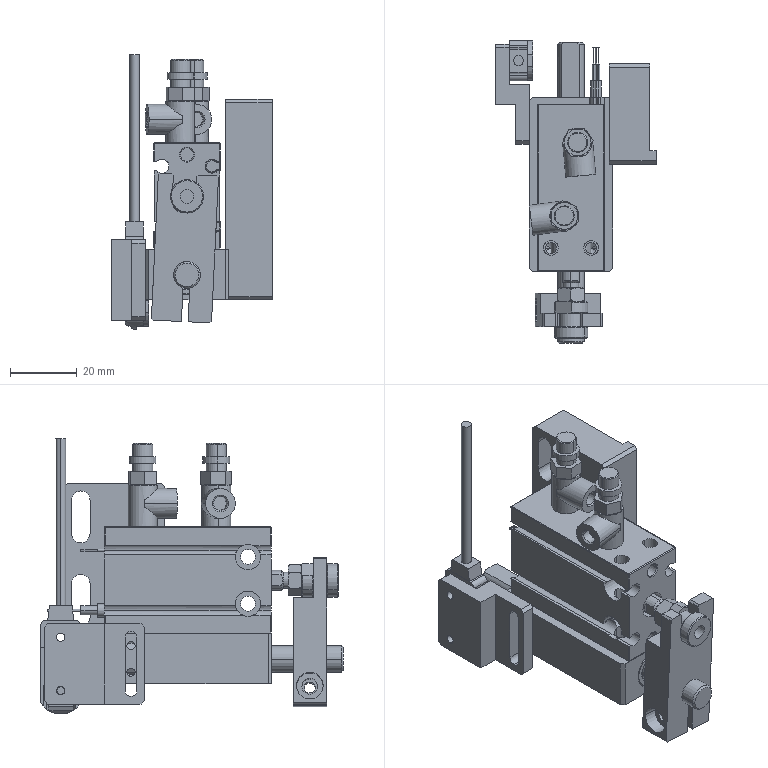Part | NX | features BREP 13 | 16 solids | 632 faces | box 48 x 90.5 x 82.2 mm | volume 79110 mm3 | plane 270 | cylinder 258 | cone 58 | torus 34 | sphere 8 | spline 4 | commonest cylinder face diameters 0.5 x28 8 x21 4.5 x20 7.6 x20 6 x16 4 x14